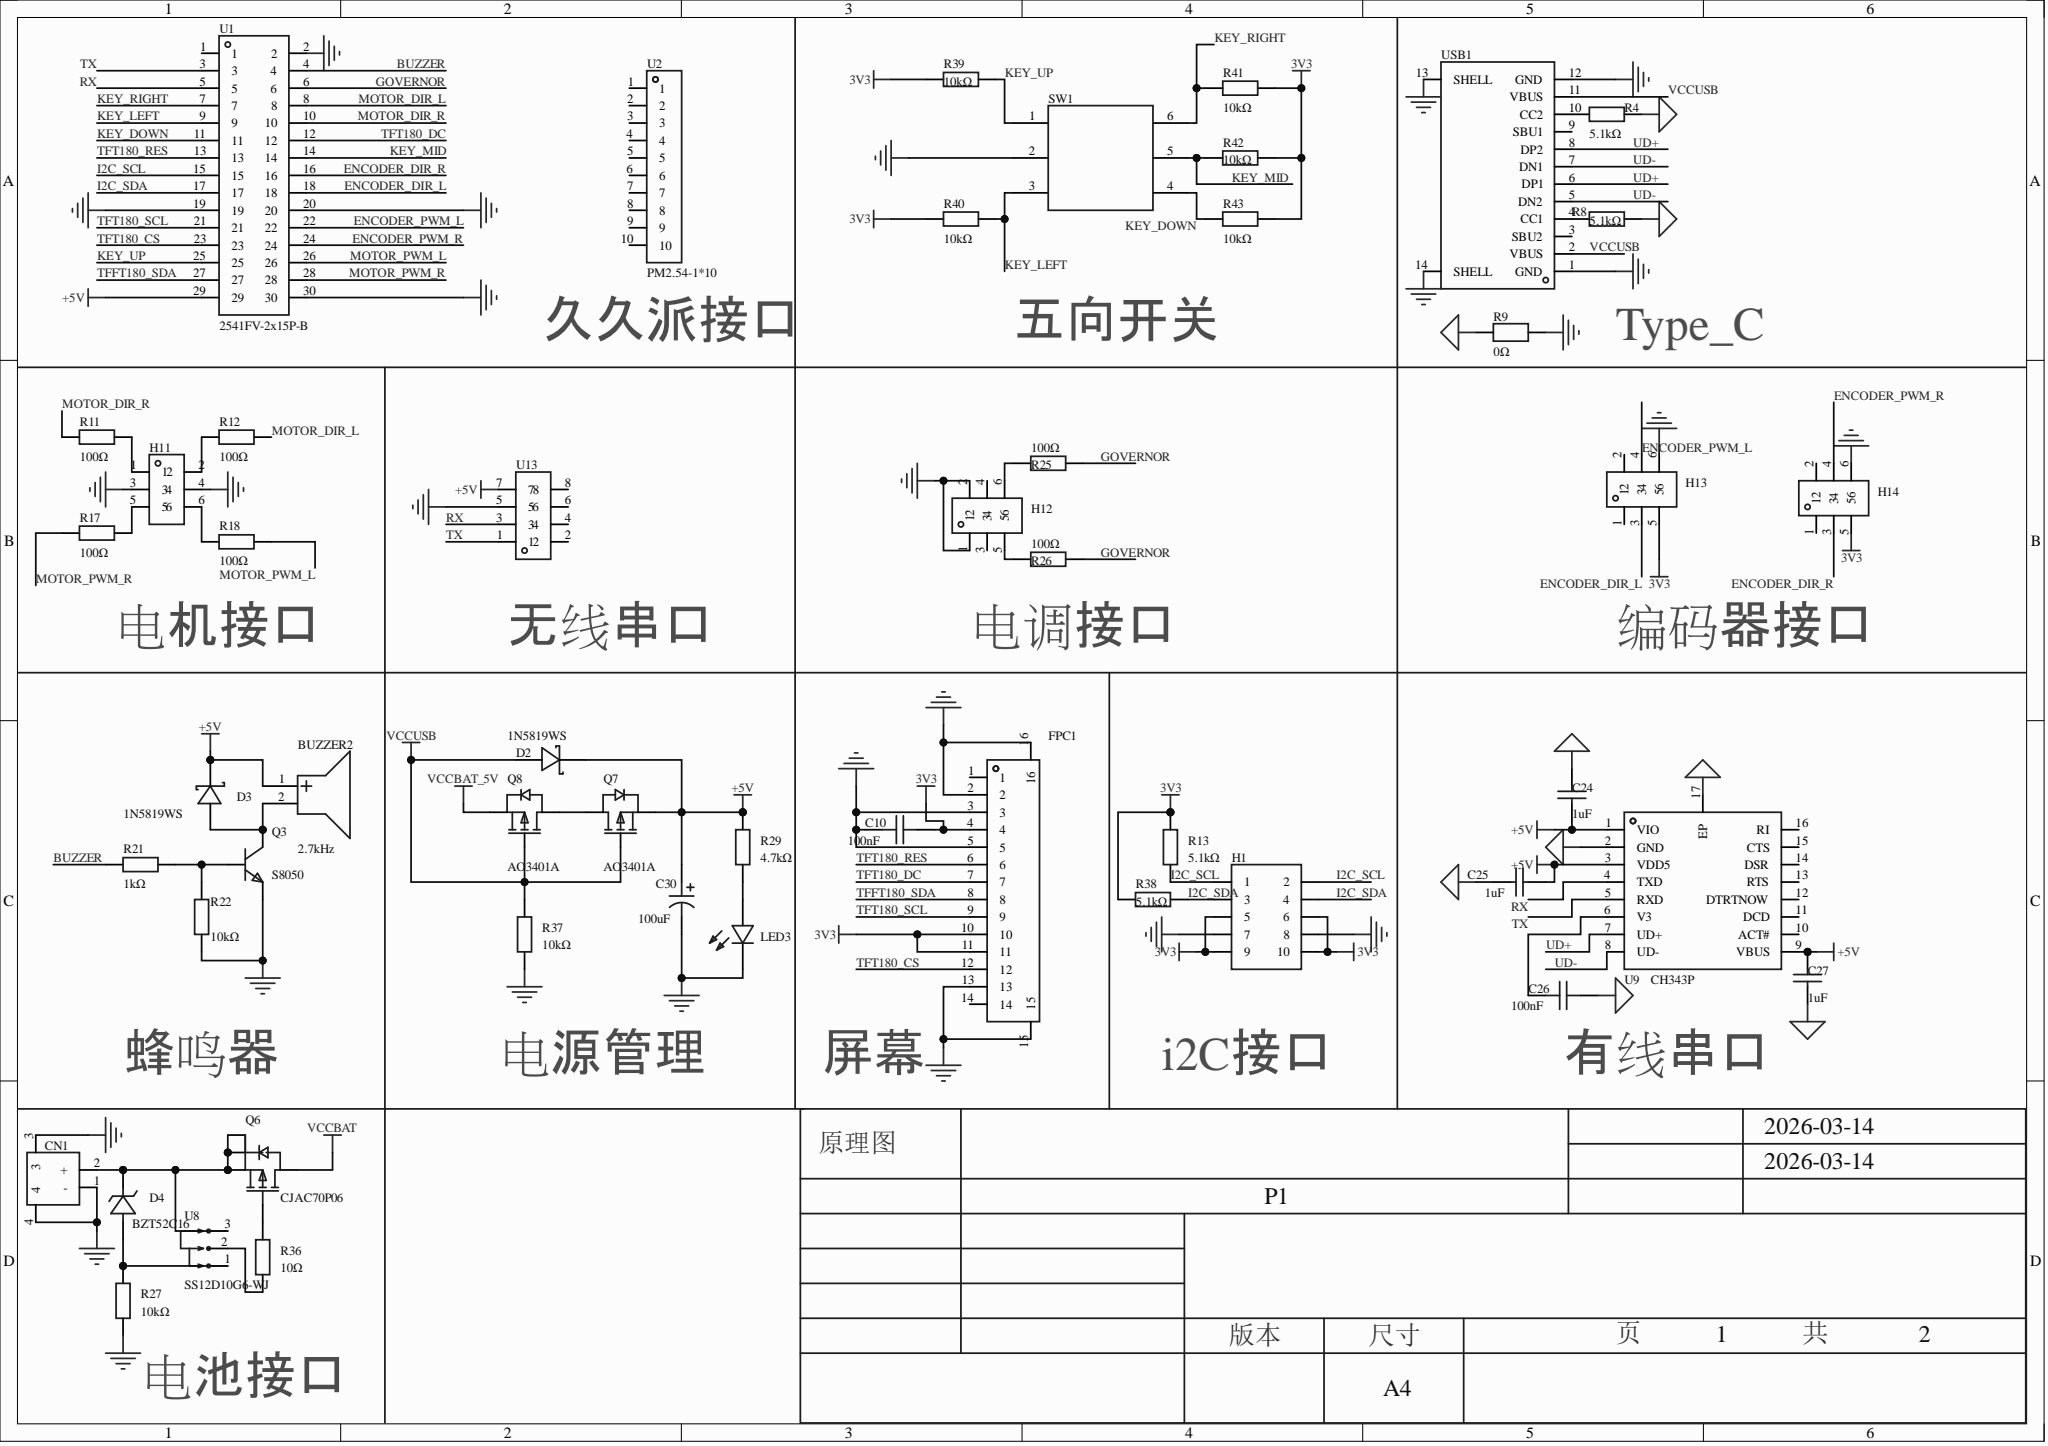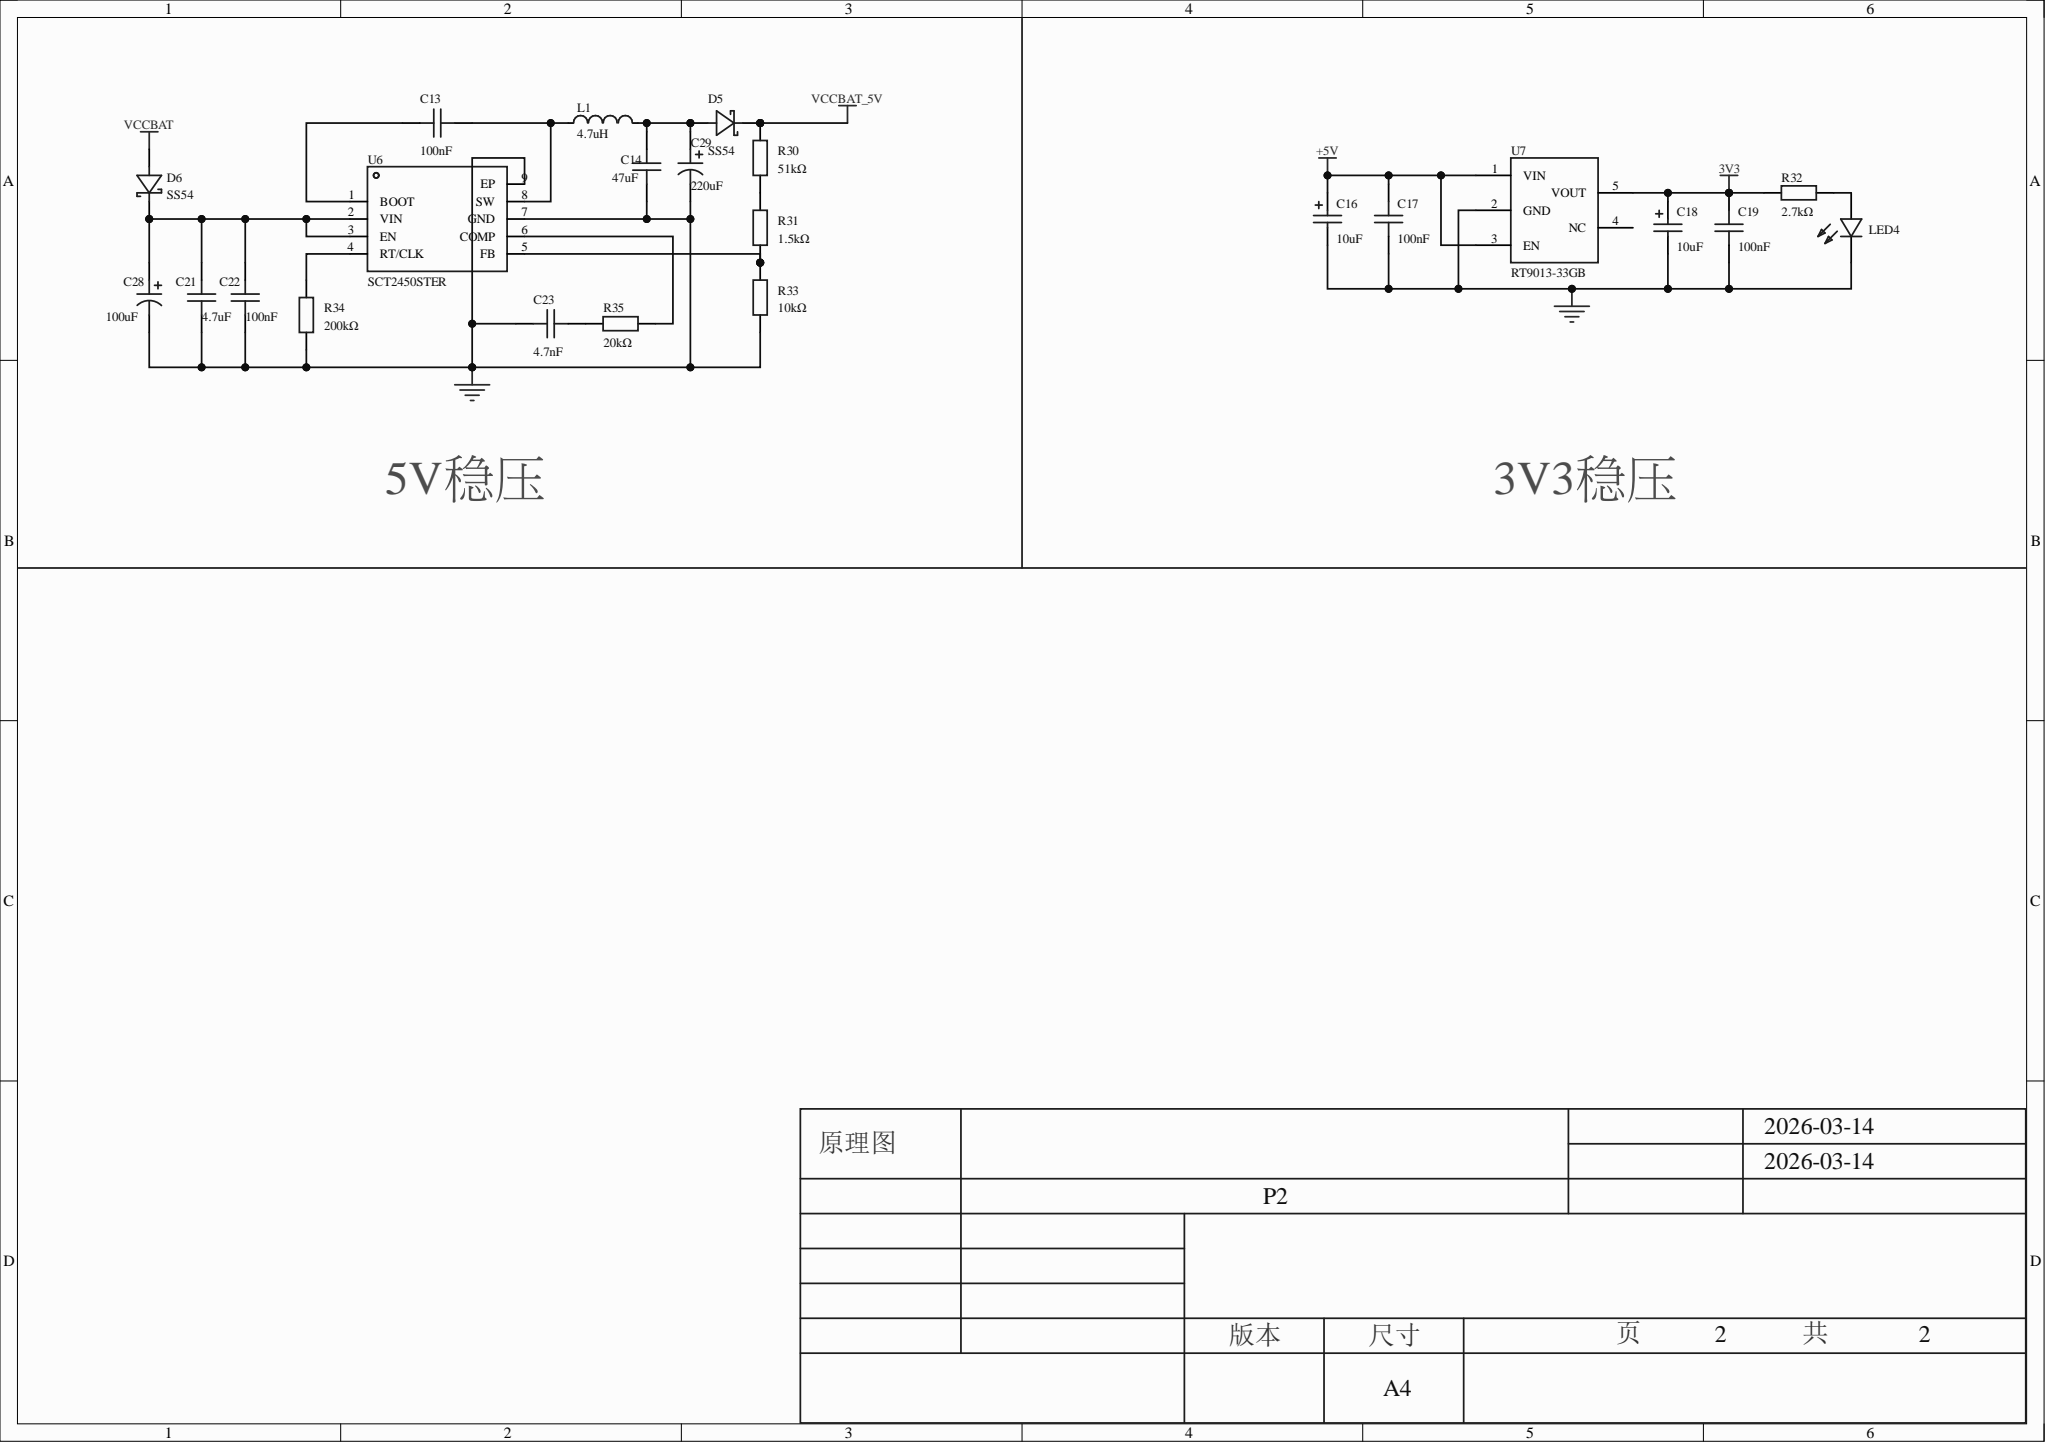Circuit board | Altium Designer | 74 parts | 60 nets
Bill of materials:
Comment,Description,Designator,Footprint,LibRef,Quantity
"2.7kHz","","BUZZER2","BUZ-SMD_GSC9032RB","GSC9032RB-16R2700","1"
"100nF","","C10, C13, C17, C19, C22, C26","C0603","CGA0603X7R104K500JT","6"
"47uF","","C14","C1206","CGA1206X5R476M250NT","1"
"10uF","","C16, C18","CAP-SMD_L3.2-W1.6-RD-C7171","TAJA106K016RNJ","2"
"4.7uF","","C21","C1206","CGA1206X5R475K350NT","1"
"4.7nF","","C23","C0603","CGA0603X7R472K500JT","1"
"1uF","","C24, C25, C27","C0805","CL21B105KBFNNNE","3"
"100uF","","C28, C30","CAP-SMD_BD6.3-L6.6-W6.6-FD-1","JVJ25V100M6x5","2"
"220uF","","C29","CAP-SMD_BD6.3-L6.6-W6.6-LS7.3-FD-H7.7","JVJ25V220M6x8","1"
"XT30PW-M30.G.Y","","CN1","CONN-TH_XT30PW-M","XT30PW-M30.G.Y","1"
"1N5819WS","","D2, D3","SOD-323_L1.8-W1.3-LS2.5-RD","1N5819WS_C191023","2"
"BZT52C16","","D4","SOD-123_L2.7-W1.6-LS3.7-RD","BZT52C16_C19077413","1"
"SS54","","D5, D6","SMA_L4.3-W2.6-LS5.0-FD","SS54_C7420369","2"
"HC-FPC-05-09-14RLTAG","","FPC1","FPC-SMD_14P-P0.50_HC-FPC-05-09-14RLTAG","HC-FPC-05-09-14RLTAG","1"
"","","H1","HDR-TH_10P-P2.54-V-F-R2-C5-S2.54","HDR-F_2.54_2x5","1"
"HX PZ2.54-2x3P TP","","H11, H12","HDR-SMD_6P-P2.54-V-M-R2-C3-LS7.2_M20-8760342","HX PZ2.54-2x3P TP","2"
"PZ254V-12-6P","","H13, H14","HDR-TH_6P-P2.54-V-M-R2-C3-S2.54","PZ254V-12-6P","2"
"4.7uH","","L1","IND-SMD_L5.4-W5.2_FXL0530","FXL0530-4R7-M","1"
"NCD0603R1","","LED3, LED4","LED0603-RD_RED","NCD0603R1_C84263","2"
"S8050","","Q3","SOT-23-3_L2.9-W1.6-P1.90-LS2.8-BR","S8050_C181158","1"
"CJAC70P06","","Q6","TDSON-8_L5.9-W5.2-P1.27-BL","CJAC70P06","1"
"AO3401A","","Q7, Q8","SOT-23_L2.9-W1.3-P1.90-LS2.4-BR","AO3401A_C347476","2"
"5.1kΩ","","R4, R8, R13, R38","R0603","0603WAF5101T5E","4"
"0Ω","","R9","R1206","FRC1206P000 TS","1"
"100Ω","","R11, R12, R17, R18, R25, R26","R0603","0603WAF1000T5E","6"
"1kΩ","","R21","R0603","0603WAF1001T5E","1"
"10kΩ","","R22, R27, R33, R37, R39, R40, R41, R42, R43","R0603","0603WAF1002T5E","9"
"4.7kΩ","","R29","R0603","0603WAF4701T5E","1"
"51kΩ","","R30","R0603","0603WAF5102T5E","1"
"1.5kΩ","","R31","R0603","0603WAF1501T5E","1"
"2.7kΩ","","R32","R0603","0603WAF2701T5E","1"
"200kΩ","","R34","R0603","0603WAF2003T5E","1"
"20kΩ","","R35","R0603","0603WAF2002T5E","1"
"10Ω","","R36","R0603","0603WAF100JT5E","1"
"7*7*5-6P-L WX","","SW1","SW-SMD_8P-L7.0-W7.0-P1.40-LS7.4-TL","7*7*5-6P-L WX","1"
"2541FV-2x15P-B","","U1","HDR-TH_30P-P2.54-V-F-R2-C15-S2.54","2541FV-2x15P-B","1"
"PM2.54-1*10","","U2","HDR-TH_10P-P2.54-V-F","PM2.54-1*10","1"
"SCT2450STER","","U6","ESOP-8_L4.9-W3.9-P1.27-LS6.0-BL-EP","SCT2450STER","1"
"RT9013-33GB","","U7","SOT-23-5_L3.0-W1.7-P0.95-LS2.8-BL","RT9013-33GB","1"
"SS12D10G6-WJ","","U8","SW-TH_3P-P4.80_HX-SS12D10G6-WJ","SS12D10G6-WJ","1"
"CH343P","","U9","TQFN-16_L3.0-W3.0-P0.50-BL-EP1.7","CH343P","1"
"5BME8-08872-204-W0","","U13","CONN-SMD_5BME8-08872-204-W0","5BME8-08872-204-W0","1"
"TYPE-C 16PIN 2MD(073)","","USB1","USB-C-SMD_TYPE-C-6PIN-2MD-073","TYPE-C 16PIN 2MD(073)","1"
Netlist (Protel format):
[
BUZZER2
BUZ-SMD_GSC9032RB
2.7kHz



]
[
C10
C0603
100nF



]
[
C13
C0603
100nF



]
[
C14
C1206
47uF



]
[
C16
CAP-SMD_L3.2-W1.6-RD-C7171
10uF



]
[
C17
C0603
100nF



]
[
C18
CAP-SMD_L3.2-W1.6-RD-C7171
10uF



]
[
C19
C0603
100nF



]
[
C21
C1206
4.7uF



]
[
C22
C0603
100nF



]
[
C23
C0603
4.7nF



]
[
C24
C0805
1uF



]
[
C25
C0805
1uF



]
[
C26
C0603
100nF



]
[
C27
C0805
1uF



]
[
C28
CAP-SMD_BD6.3-L6.6-W6.6-FD-1
100uF



]
[
C29
CAP-SMD_BD6.3-L6.6-W6.6-LS7.3-FD-H7.7
220uF



]
[
C30
CAP-SMD_BD6.3-L6.6-W6.6-FD-1
100uF



]
[
CN1
CONN-TH_XT30PW-M
XT30PW-M30.G.Y



]
[
D2
SOD-323_L1.8-W1.3-LS2.5-RD
1N5819WS



]
[
D3
SOD-323_L1.8-W1.3-LS2.5-RD
1N5819WS



]
[
D4
SOD-123_L2.7-W1.6-LS3.7-RD
BZT52C16



]
[
D5
SMA_L4.3-W2.6-LS5.0-FD
SS54



]
[
D6
SMA_L4.3-W2.6-LS5.0-FD
SS54



]
[
FPC1
FPC-SMD_14P-P0.50_HC-FPC-05-09-14RLTAG
HC-FPC-05-09-14RLTAG



]
[
H1
HDR-TH_10P-P2.54-V-F-R2-C5-S2.54




]
[
H11
HDR-SMD_6P-P2.54-V-M-R2-C3-LS7.2_M20-8760342
HX PZ2.54-2x3P TP



]
[
H12
HDR-SMD_6P-P2.54-V-M-R2-C3-LS7.2_M20-8760342
HX PZ2.54-2x3P TP



]
[
H13
HDR-TH_6P-P2.54-V-M-R2-C3-S2.54
PZ254V-12-6P



]
[
H14
HDR-TH_6P-P2.54-V-M-R2-C3-S2.54
PZ254V-12-6P



]
[
L1
IND-SMD_L5.4-W5.2_FXL0530
4.7uH



]
[
LED3
LED0603-RD_RED
NCD0603R1



]
[
LED4
LED0603-RD_RED
NCD0603R1



]
[
Q3
SOT-23-3_L2.9-W1.6-P1.90-LS2.8-BR
S8050



]
[
Q6
TDSON-8_L5.9-W5.2-P1.27-BL
CJAC70P06



]
[
Q7
SOT-23_L2.9-W1.3-P1.90-LS2.4-BR
AO3401A



]
[
Q8
SOT-23_L2.9-W1.3-P1.90-LS2.4-BR
AO3401A



]
[
R4
R0603
5.1kΩ



]
[
R8
R0603
5.1kΩ



]
[
R9
R1206
0Ω



]
[
R11
R0603
100Ω



]
[
R12
R0603
100Ω



]
[
R13
R0603
5.1kΩ



]
[
R17
R0603
100Ω



]
[
R18
R0603
100Ω



]
[
R21
R0603
1kΩ



]
[
R22
R0603
10kΩ



]
[
R25
R0603
100Ω



]
[
R26
R0603
100Ω



]
[
R27
R0603
10kΩ



]
[
R29
R0603
4.7kΩ



]
[
R30
R0603
51kΩ



]
[
R31
R0603
1.5kΩ



]
[
R32
R0603
2.7kΩ



]
[
R33
R0603
10kΩ



]
[
R34
R0603
200kΩ



]
[
R35
R0603
20kΩ



]
[
R36
R0603
10Ω



]
[
R37
R0603
10kΩ



]
[
R38
R0603
5.1kΩ



]
[
R39
R0603
10kΩ



]
[
R40
R0603
10kΩ



]
[
R41
R0603
10kΩ



]
[
R42
R0603
10kΩ



]
[
R43
R0603
10kΩ



]
[
SW1
SW-SMD_8P-L7.0-W7.0-P1.40-LS7.4-TL
7*7*5-6P-L WX



]
[
U1
HDR-TH_30P-P2.54-V-F-R2-C15-S2.54
2541FV-2x15P-B



]
[
U2
HDR-TH_10P-P2.54-V-F
PM2.54-1*10



]
[
U6
ESOP-8_L4.9-W3.9-P1.27-LS6.0-BL-EP
SCT2450STER



]
[
U7
SOT-23-5_L3.0-W1.7-P0.95-LS2.8-BL
RT9013-33GB



]
[
U8
SW-TH_3P-P4.80_HX-SS12D10G6-WJ
SS12D10G6-WJ



]
[
U9
TQFN-16_L3.0-W3.0-P0.50-BL-EP1.7
CH343P



]
[
U13
CONN-SMD_5BME8-08872-204-W0
5BME8-08872-204-W0



]
[
USB1
USB-C-SMD_TYPE-C-6PIN-2MD-073
TYPE-C 16PIN 2MD(073)



]
(
VCCUSB
D2-2
Q7-1
Q8-1
R37-2
USB1-2
USB1-11
)
(
VCCBAT_5V
D5-2
Q8-2
R30-2
)
(
VCCBAT
D6-1
Q6-5
)
(
UD-
U9-8
USB1-5
USB1-7
)
(
UD+
U9-7
USB1-6
USB1-8
)
(
TX
U1-3
U9-5
U13-1
)
(
TFT180_SCL
FPC1-9
U1-21
)
(
TFT180_RES
FPC1-6
U1-13
)
(
TFT180_DC
FPC1-7
U1-12
)
(
TFT180_CS
FPC1-12
U1-23
)
(
TFFT180_SDA
FPC1-8
U1-27
)
(
RX
U1-5
U9-4
U13-3
)
(
NetR36_1
R36-1
U8-2
)
(
NetR35_2
R35-2
U6-6
)
(
NetR34_2
R34-2
U6-4
)
(
NetR31_1
R31-1
R33-2
U6-5
)
(
NetR30_1
R30-1
R31-2
)
(
NetR8_1
R8-1
USB1-4
)
(
NetR4_1
R4-1
USB1-10
)
(
NetQ7_3
Q7-3
Q8-3
)
(
NetQ6_4
Q6-4
R36-2
)
(
NetQ3_1
Q3-1
R21-2
R22-1
)
(
NetLED4_2
LED4-2
R32-2
)
(
NetLED3_2
LED3-2
R29-1
)
(
NetH12_6
H12-6
R25-1
)
(
NetH12_5
H12-5
R26-1
)
(
NetH11_6
H11-6
R18-1
)
(
NetH11_5
H11-5
R17-2
)
(
NetH11_2
H11-2
R12-1
)
(
NetH11_1
H11-1
R11-2
)
(
NetD4_2
D4-2
R27-2
U8-1
)
(
NetCN1_2
CN1-2
D4-1
Q6-1
Q6-2
Q6-3
U8-3
)
(
NetC26_1
C26-1
U9-6
)
(
NetC23_2
C23-2
R35-1
)
(
NetC21_2
C21-2
C22-2
C28-1
D6-2
U6-2
U6-3
)
(
NetC14_2
C14-2
C29-1
D5-1
L1-2
)
(
NetC13_2
C13-2
U6-1
)
(
NetC13_1
C13-1
L1-1
U6-8
)
(
NetBUZZER2_2
BUZZER2-2
D3-2
Q3-3
)
(
MOTOR_PWM_R
R17-1
U1-28
)
(
MOTOR_PWM_L
R18-2
U1-26
)
(
MOTOR_DIR_R
R11-1
U1-10
)
(
MOTOR_DIR_L
R12-2
U1-8
)
(
KEY_UP
R39-2
SW1-1
U1-25
)
(
KEY_RIGHT
R41-1
SW1-6
U1-7
)
(
KEY_MID
R42-1
SW1-5
U1-14
)
(
KEY_LEFT
R40-2
SW1-3
U1-9
)
(
KEY_DOWN
R43-1
SW1-4
U1-11
)
(
I2C_SDA
H1-3
H1-4
R38-1
U1-17
)
(
I2C_SCL
H1-1
H1-2
R13-1
U1-15
)
(
GOVERNOR
R25-2
R26-2
U1-6
)
(
GND
C10-1
C14-1
C16-2
C17-2
C18-2
C19-2
C21-1
C22-1
C23-1
C28-2
C29-2
C30-2
CN1-1
CN1-3
CN1-4
FPC1-2
FPC1-3
FPC1-5
FPC1-13
FPC1-15
FPC1-16
H1-7
H1-8
H11-3
H11-4
H12-1
H12-2
H13-6
H14-6
LED3-1
LED4-1
Q3-2
R9-2
R22-2
R27-1
R33-1
R34-1
R37-1
SW1-2
U1-2
U1-19
U1-20
U1-30
U6-7
U6-9
U7-2
U13-5
USB1-1
USB1-12
USB1-13
USB1-14
)
(
ENCODER_PWM_R
H14-4
U1-24
)
(
ENCODER_PWM_L
H13-4
U1-22
)
(
ENCODER_DIR_R
H14-3
U1-16
)
(
ENCODER_DIR_L
H13-3
U1-18
)
(
BUZZER
R21-1
U1-4
)
(
AGND
C24-2
C25-2
C26-2
C27-1
R4-2
R8-2
R9-1
U9-2
U9-17
)
(
+5V
BUZZER2-1
C16-1
C17-1
C24-1
C25-1
C27-2
C30-1
D2-1
D3-1
Q7-2
R29-2
U1-29
U7-1
U7-3
U9-1
U9-3
U9-9
U13-7
)
(
3V3
C10-2
C18-1
C19-1
FPC1-4
FPC1-10
FPC1-11
H1-5
H1-6
H1-9
H1-10
H13-5
H14-5
R13-2
R32-1
R38-2
R39-1
R40-1
R41-2
R42-2
R43-2
U7-5
)